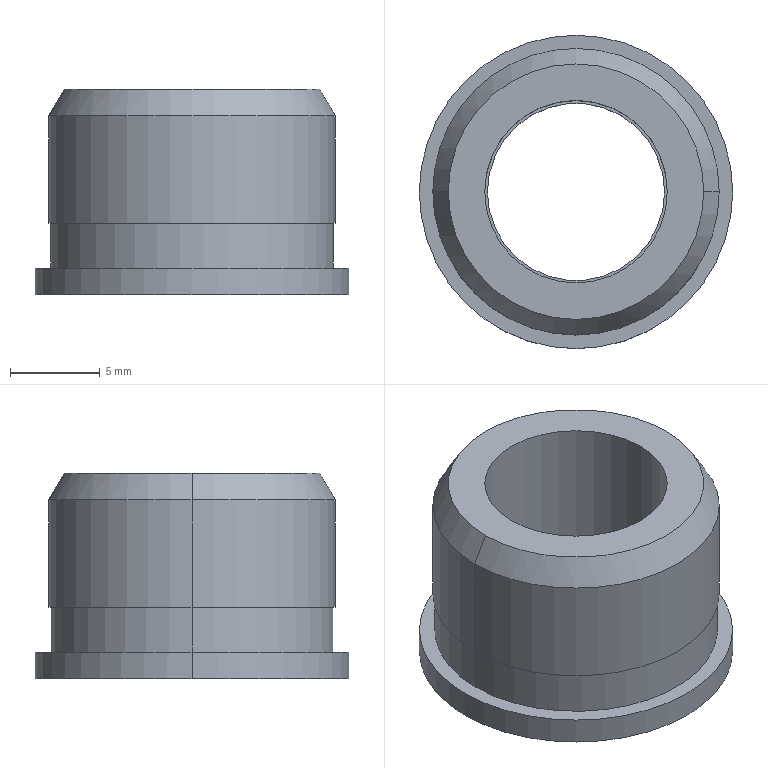Part | SolidWorks | features BaseBody 1 | 1 solid | 17 faces | box 17.5 x 17.5 x 11.5 mm | volume 1402 mm3 | cylinder 10 | plane 5 | cone 2 | commonest cylinder face diameters 9.9 x2 10.2 x2 15.8 x2 16 x2 17.5 x2
STEP:
#1=CARTESIAN_POINT('',(485.487,37.715,-16.134));
#2=VERTEX_POINT('',#1);
#3=CARTESIAN_POINT('',(475.587,37.715,-16.134));
#4=VERTEX_POINT('',#3);
#5=CARTESIAN_POINT('',(480.537,37.715,-16.134));
#6=DIRECTION('',(0.000000013,0.,-1.));
#7=DIRECTION('',(1.,0.,0.000000013));
#8=AXIS2_PLACEMENT_3D('',#5,#6,#7);
#9=CIRCLE('',#8,4.95);
#10=EDGE_CURVE('',#2,#4,#9,.T.);
#11=ORIENTED_EDGE('',*,*,#10,.T.);
#12=CARTESIAN_POINT('',(475.587,37.715,-13.134));
#13=VERTEX_POINT('',#12);
#14=CARTESIAN_POINT('',(475.587,37.715,-16.134));
#15=DIRECTION('',(-0.000000013,0.,1.));
#16=VECTOR('',#15,1000.);
#17=LINE('',#14,#16);
#18=EDGE_CURVE('',#4,#13,#17,.T.);
#19=ORIENTED_EDGE('',*,*,#18,.T.);
#20=CARTESIAN_POINT('',(485.487,37.715,-13.134));
#21=VERTEX_POINT('',#20);
#22=CARTESIAN_POINT('',(480.537,37.715,-13.134));
#23=DIRECTION('',(-0.000000013,0.,1.));
#24=DIRECTION('',(1.,0.,0.000000013));
#25=AXIS2_PLACEMENT_3D('',#22,#23,#24);
#26=CIRCLE('',#25,4.95);
#27=EDGE_CURVE('',#13,#21,#26,.T.);
#28=ORIENTED_EDGE('',*,*,#27,.T.);
#29=CARTESIAN_POINT('',(485.487,37.715,-16.134));
#30=DIRECTION('',(-0.000000013,0.,1.));
#31=VECTOR('',#30,1000.);
#32=LINE('',#29,#31);
#33=EDGE_CURVE('',#2,#21,#32,.T.);
#34=ORIENTED_EDGE('',*,*,#33,.F.);
#35=EDGE_LOOP('',(#11,#19,#28,#34));
#36=FACE_OUTER_BOUND('',#35,.T.);
#37=CARTESIAN_POINT('',(480.537,37.715,-16.134));
#38=DIRECTION('',(-0.000000013,0.,1.));
#39=DIRECTION('',(1.,0.,0.000000013));
#40=AXIS2_PLACEMENT_3D('',#37,#38,#39);
#41=CYLINDRICAL_SURFACE('',#40,4.95);
#42=ADVANCED_FACE('',(#36),#41,.F.);
#43=CARTESIAN_POINT('',(489.287,37.715,-16.134));
#44=VERTEX_POINT('',#43);
#45=CARTESIAN_POINT('',(471.787,37.715,-16.134));
#46=VERTEX_POINT('',#45);
#47=CARTESIAN_POINT('',(480.537,37.715,-16.134));
#48=DIRECTION('',(-0.000000013,0.,1.));
#49=DIRECTION('',(1.,0.,0.000000013));
#50=AXIS2_PLACEMENT_3D('',#47,#48,#49);
#51=CIRCLE('',#50,8.75);
#52=EDGE_CURVE('',#44,#46,#51,.T.);
#53=ORIENTED_EDGE('',*,*,#52,.T.);
#54=CARTESIAN_POINT('',(471.787,37.715,-14.634));
#55=VERTEX_POINT('',#54);
#56=CARTESIAN_POINT('',(471.787,37.715,-16.134));
#57=DIRECTION('',(-0.000000013,0.,1.));
#58=VECTOR('',#57,1000.);
#59=LINE('',#56,#58);
#60=EDGE_CURVE('',#46,#55,#59,.T.);
#61=ORIENTED_EDGE('',*,*,#60,.T.);
#62=CARTESIAN_POINT('',(489.287,37.715,-14.634));
#63=VERTEX_POINT('',#62);
#64=CARTESIAN_POINT('',(480.537,37.715,-14.634));
#65=DIRECTION('',(-0.000000013,0.,1.));
#66=DIRECTION('',(1.,0.,0.000000013));
#67=AXIS2_PLACEMENT_3D('',#64,#65,#66);
#68=CIRCLE('',#67,8.75);
#69=EDGE_CURVE('',#63,#55,#68,.T.);
#70=ORIENTED_EDGE('',*,*,#69,.F.);
#71=CARTESIAN_POINT('',(489.287,37.715,-16.134));
#72=DIRECTION('',(-0.000000013,0.,1.));
#73=VECTOR('',#72,1000.);
#74=LINE('',#71,#73);
#75=EDGE_CURVE('',#44,#63,#74,.T.);
#76=ORIENTED_EDGE('',*,*,#75,.F.);
#77=EDGE_LOOP('',(#53,#61,#70,#76));
#78=FACE_OUTER_BOUND('',#77,.T.);
#79=CARTESIAN_POINT('',(480.537,37.715,-16.134));
#80=DIRECTION('',(-0.000000013,0.,1.));
#81=DIRECTION('',(1.,0.,0.000000013));
#82=AXIS2_PLACEMENT_3D('',#79,#80,#81);
#83=CYLINDRICAL_SURFACE('',#82,8.75);
#84=ADVANCED_FACE('',(#78),#83,.T.);
#85=CARTESIAN_POINT('',(475.437,37.715,-13.134));
#86=VERTEX_POINT('',#85);
#87=CARTESIAN_POINT('',(485.637,37.715,-13.134));
#88=VERTEX_POINT('',#87);
#89=CARTESIAN_POINT('',(480.537,37.715,-13.134));
#90=DIRECTION('',(-0.000000013,0.,1.));
#91=DIRECTION('',(1.,0.,0.000000013));
#92=AXIS2_PLACEMENT_3D('',#89,#90,#91);
#93=CIRCLE('',#92,5.1);
#94=EDGE_CURVE('',#86,#88,#93,.T.);
#95=ORIENTED_EDGE('',*,*,#94,.F.);
#96=CARTESIAN_POINT('',(475.437,37.715,-4.634));
#97=VERTEX_POINT('',#96);
#98=CARTESIAN_POINT('',(475.437,37.715,-13.134));
#99=DIRECTION('',(-0.000000013,0.,1.));
#100=VECTOR('',#99,1000.);
#101=LINE('',#98,#100);
#102=EDGE_CURVE('',#86,#97,#101,.T.);
#103=ORIENTED_EDGE('',*,*,#102,.T.);
#104=CARTESIAN_POINT('',(485.637,37.715,-4.634));
#105=VERTEX_POINT('',#104);
#106=CARTESIAN_POINT('',(480.537,37.715,-4.634));
#107=DIRECTION('',(-0.000000013,0.,1.));
#108=DIRECTION('',(1.,0.,0.000000013));
#109=AXIS2_PLACEMENT_3D('',#106,#107,#108);
#110=CIRCLE('',#109,5.1);
#111=EDGE_CURVE('',#97,#105,#110,.T.);
#112=ORIENTED_EDGE('',*,*,#111,.T.);
#113=CARTESIAN_POINT('',(485.637,37.715,-13.134));
#114=DIRECTION('',(-0.000000013,0.,1.));
#115=VECTOR('',#114,1000.);
#116=LINE('',#113,#115);
#117=EDGE_CURVE('',#88,#105,#116,.T.);
#118=ORIENTED_EDGE('',*,*,#117,.F.);
#119=EDGE_LOOP('',(#95,#103,#112,#118));
#120=FACE_OUTER_BOUND('',#119,.T.);
#121=CARTESIAN_POINT('',(480.537,37.715,-13.134));
#122=DIRECTION('',(-0.000000013,0.,1.));
#123=DIRECTION('',(1.,0.,0.000000013));
#124=AXIS2_PLACEMENT_3D('',#121,#122,#123);
#125=CYLINDRICAL_SURFACE('',#124,5.1);
#126=ADVANCED_FACE('',(#120),#125,.F.);
#127=CARTESIAN_POINT('',(472.637,37.715,-14.634));
#128=VERTEX_POINT('',#127);
#129=CARTESIAN_POINT('',(488.437,37.715,-14.634));
#130=VERTEX_POINT('',#129);
#131=CARTESIAN_POINT('',(480.537,37.715,-14.634));
#132=DIRECTION('',(0.000000013,0.,-1.));
#133=DIRECTION('',(1.,0.,0.000000013));
#134=AXIS2_PLACEMENT_3D('',#131,#132,#133);
#135=CIRCLE('',#134,7.9);
#136=EDGE_CURVE('',#128,#130,#135,.T.);
#137=ORIENTED_EDGE('',*,*,#136,.F.);
#138=CARTESIAN_POINT('',(472.637,37.715,-12.134));
#139=VERTEX_POINT('',#138);
#140=CARTESIAN_POINT('',(472.637,37.715,-14.634));
#141=DIRECTION('',(-0.000000013,0.,1.));
#142=VECTOR('',#141,1000.);
#143=LINE('',#140,#142);
#144=EDGE_CURVE('',#128,#139,#143,.T.);
#145=ORIENTED_EDGE('',*,*,#144,.T.);
#146=CARTESIAN_POINT('',(488.437,37.715,-12.134));
#147=VERTEX_POINT('',#146);
#148=CARTESIAN_POINT('',(480.537,37.715,-12.134));
#149=DIRECTION('',(-0.000000013,0.,1.));
#150=DIRECTION('',(1.,0.,0.000000013));
#151=AXIS2_PLACEMENT_3D('',#148,#149,#150);
#152=CIRCLE('',#151,7.9);
#153=EDGE_CURVE('',#147,#139,#152,.T.);
#154=ORIENTED_EDGE('',*,*,#153,.F.);
#155=CARTESIAN_POINT('',(488.437,37.715,-14.634));
#156=DIRECTION('',(-0.000000013,0.,1.));
#157=VECTOR('',#156,1000.);
#158=LINE('',#155,#157);
#159=EDGE_CURVE('',#130,#147,#158,.T.);
#160=ORIENTED_EDGE('',*,*,#159,.F.);
#161=EDGE_LOOP('',(#137,#145,#154,#160));
#162=FACE_OUTER_BOUND('',#161,.T.);
#163=CARTESIAN_POINT('',(480.537,37.715,-14.634));
#164=DIRECTION('',(-0.000000013,0.,1.));
#165=DIRECTION('',(1.,0.,0.000000013));
#166=AXIS2_PLACEMENT_3D('',#163,#164,#165);
#167=CYLINDRICAL_SURFACE('',#166,7.9);
#168=ADVANCED_FACE('',(#162),#167,.T.);
#169=CARTESIAN_POINT('',(487.671,37.715,-4.634));
#170=VERTEX_POINT('',#169);
#171=CARTESIAN_POINT('',(473.403,37.715,-4.634));
#172=VERTEX_POINT('',#171);
#173=CARTESIAN_POINT('',(480.537,37.715,-4.634));
#174=DIRECTION('',(-0.000000013,0.,1.));
#175=DIRECTION('',(-1.,0.,-0.000000013));
#176=AXIS2_PLACEMENT_3D('',#173,#174,#175);
#177=CIRCLE('',#176,7.134);
#178=EDGE_CURVE('',#170,#172,#177,.T.);
#179=ORIENTED_EDGE('',*,*,#178,.F.);
#180=CARTESIAN_POINT('',(488.537,37.715,-6.134));
#181=VERTEX_POINT('',#180);
#182=CARTESIAN_POINT('',(488.537,37.715,-6.134));
#183=DIRECTION('',(0.5,0.,-0.866));
#184=VECTOR('',#183,1000.);
#185=LINE('',#182,#184);
#186=EDGE_CURVE('',#170,#181,#185,.T.);
#187=ORIENTED_EDGE('',*,*,#186,.T.);
#188=CARTESIAN_POINT('',(472.537,37.715,-6.134));
#189=VERTEX_POINT('',#188);
#190=CARTESIAN_POINT('',(480.537,37.715,-6.134));
#191=DIRECTION('',(0.000000013,0.,-1.));
#192=DIRECTION('',(0.,1.,0.));
#193=AXIS2_PLACEMENT_3D('',#190,#191,#192);
#194=CIRCLE('',#193,8.);
#195=EDGE_CURVE('',#189,#181,#194,.T.);
#196=ORIENTED_EDGE('',*,*,#195,.F.);
#197=CARTESIAN_POINT('',(472.537,37.715,-6.134));
#198=DIRECTION('',(-0.5,0.,-0.866));
#199=VECTOR('',#198,1000.);
#200=LINE('',#197,#199);
#201=EDGE_CURVE('',#172,#189,#200,.T.);
#202=ORIENTED_EDGE('',*,*,#201,.F.);
#203=EDGE_LOOP('',(#179,#187,#196,#202));
#204=FACE_OUTER_BOUND('',#203,.T.);
#205=CARTESIAN_POINT('',(480.537,37.715,-6.134));
#206=DIRECTION('',(0.000000013,0.,-1.));
#207=DIRECTION('',(-1.,0.,-0.000000013));
#208=AXIS2_PLACEMENT_3D('',#205,#206,#207);
#209=CONICAL_SURFACE('',#208,8.,0.5236);
#210=ADVANCED_FACE('',(#204),#209,.T.);
#211=CARTESIAN_POINT('',(488.537,37.715,-12.134));
#212=VERTEX_POINT('',#211);
#213=CARTESIAN_POINT('',(472.537,37.715,-12.134));
#214=VERTEX_POINT('',#213);
#215=CARTESIAN_POINT('',(480.537,37.715,-12.134));
#216=DIRECTION('',(-0.000000013,0.,1.));
#217=DIRECTION('',(1.,0.,0.000000013));
#218=AXIS2_PLACEMENT_3D('',#215,#216,#217);
#219=CIRCLE('',#218,8.);
#220=EDGE_CURVE('',#212,#214,#219,.T.);
#221=ORIENTED_EDGE('',*,*,#220,.T.);
#222=CARTESIAN_POINT('',(472.537,37.715,-12.134));
#223=DIRECTION('',(-0.000000013,0.,1.));
#224=VECTOR('',#223,1000.);
#225=LINE('',#222,#224);
#226=EDGE_CURVE('',#214,#189,#225,.T.);
#227=ORIENTED_EDGE('',*,*,#226,.T.);
#228=ORIENTED_EDGE('',*,*,#195,.T.);
#229=CARTESIAN_POINT('',(488.537,37.715,-12.134));
#230=DIRECTION('',(-0.000000013,0.,1.));
#231=VECTOR('',#230,1000.);
#232=LINE('',#229,#231);
#233=EDGE_CURVE('',#212,#181,#232,.T.);
#234=ORIENTED_EDGE('',*,*,#233,.F.);
#235=EDGE_LOOP('',(#221,#227,#228,#234));
#236=FACE_OUTER_BOUND('',#235,.T.);
#237=CARTESIAN_POINT('',(480.537,37.715,-12.134));
#238=DIRECTION('',(-0.000000013,0.,1.));
#239=DIRECTION('',(1.,0.,0.000000013));
#240=AXIS2_PLACEMENT_3D('',#237,#238,#239);
#241=CYLINDRICAL_SURFACE('',#240,8.);
#242=ADVANCED_FACE('',(#236),#241,.T.);
#243=ORIENTED_EDGE('',*,*,#10,.F.);
#244=CARTESIAN_POINT('',(480.537,37.715,-16.134));
#245=DIRECTION('',(0.000000013,0.,-1.));
#246=DIRECTION('',(1.,0.,0.000000013));
#247=AXIS2_PLACEMENT_3D('',#244,#245,#246);
#248=CIRCLE('',#247,4.95);
#249=EDGE_CURVE('',#4,#2,#248,.T.);
#250=ORIENTED_EDGE('',*,*,#249,.F.);
#251=EDGE_LOOP('',(#243,#250));
#252=FACE_BOUND('',#251,.T.);
#253=ORIENTED_EDGE('',*,*,#52,.F.);
#254=CARTESIAN_POINT('',(480.537,37.715,-16.134));
#255=DIRECTION('',(-0.000000013,0.,1.));
#256=DIRECTION('',(1.,0.,0.000000013));
#257=AXIS2_PLACEMENT_3D('',#254,#255,#256);
#258=CIRCLE('',#257,8.75);
#259=EDGE_CURVE('',#46,#44,#258,.T.);
#260=ORIENTED_EDGE('',*,*,#259,.F.);
#261=EDGE_LOOP('',(#253,#260));
#262=FACE_OUTER_BOUND('',#261,.T.);
#263=CARTESIAN_POINT('',(489.641,28.615,-16.134));
#264=DIRECTION('',(-0.000000013,0.,1.));
#265=DIRECTION('',(0.,1.,0.));
#266=AXIS2_PLACEMENT_3D('',#263,#264,#265);
#267=PLANE('',#266);
#268=ADVANCED_FACE('',(#252,#262),#267,.F.);
#269=ORIENTED_EDGE('',*,*,#18,.F.);
#270=ORIENTED_EDGE('',*,*,#249,.T.);
#271=ORIENTED_EDGE('',*,*,#33,.T.);
#272=CARTESIAN_POINT('',(480.537,37.715,-13.134));
#273=DIRECTION('',(-0.000000013,0.,1.));
#274=DIRECTION('',(1.,0.,0.000000013));
#275=AXIS2_PLACEMENT_3D('',#272,#273,#274);
#276=CIRCLE('',#275,4.95);
#277=EDGE_CURVE('',#21,#13,#276,.T.);
#278=ORIENTED_EDGE('',*,*,#277,.T.);
#279=EDGE_LOOP('',(#269,#270,#271,#278));
#280=FACE_OUTER_BOUND('',#279,.T.);
#281=CARTESIAN_POINT('',(480.537,37.715,-16.134));
#282=DIRECTION('',(-0.000000013,0.,1.));
#283=DIRECTION('',(1.,0.,0.000000013));
#284=AXIS2_PLACEMENT_3D('',#281,#282,#283);
#285=CYLINDRICAL_SURFACE('',#284,4.95);
#286=ADVANCED_FACE('',(#280),#285,.F.);
#287=ORIENTED_EDGE('',*,*,#60,.F.);
#288=ORIENTED_EDGE('',*,*,#259,.T.);
#289=ORIENTED_EDGE('',*,*,#75,.T.);
#290=CARTESIAN_POINT('',(480.537,37.715,-14.634));
#291=DIRECTION('',(-0.000000013,0.,1.));
#292=DIRECTION('',(1.,0.,0.000000013));
#293=AXIS2_PLACEMENT_3D('',#290,#291,#292);
#294=CIRCLE('',#293,8.75);
#295=EDGE_CURVE('',#55,#63,#294,.T.);
#296=ORIENTED_EDGE('',*,*,#295,.F.);
#297=EDGE_LOOP('',(#287,#288,#289,#296));
#298=FACE_OUTER_BOUND('',#297,.T.);
#299=CARTESIAN_POINT('',(480.537,37.715,-16.134));
#300=DIRECTION('',(-0.000000013,0.,1.));
#301=DIRECTION('',(1.,0.,0.000000013));
#302=AXIS2_PLACEMENT_3D('',#299,#300,#301);
#303=CYLINDRICAL_SURFACE('',#302,8.75);
#304=ADVANCED_FACE('',(#298),#303,.T.);
#305=ORIENTED_EDGE('',*,*,#277,.F.);
#306=ORIENTED_EDGE('',*,*,#27,.F.);
#307=EDGE_LOOP('',(#305,#306));
#308=FACE_BOUND('',#307,.T.);
#309=CARTESIAN_POINT('',(480.537,37.715,-13.134));
#310=DIRECTION('',(-0.000000013,0.,1.));
#311=DIRECTION('',(1.,0.,0.000000013));
#312=AXIS2_PLACEMENT_3D('',#309,#310,#311);
#313=CIRCLE('',#312,5.1);
#314=EDGE_CURVE('',#88,#86,#313,.T.);
#315=ORIENTED_EDGE('',*,*,#314,.T.);
#316=ORIENTED_EDGE('',*,*,#94,.T.);
#317=EDGE_LOOP('',(#315,#316));
#318=FACE_OUTER_BOUND('',#317,.T.);
#319=CARTESIAN_POINT('',(485.841,32.411,-13.134));
#320=DIRECTION('',(-0.000000013,0.,1.));
#321=DIRECTION('',(0.,1.,0.));
#322=AXIS2_PLACEMENT_3D('',#319,#320,#321);
#323=PLANE('',#322);
#324=ADVANCED_FACE('',(#308,#318),#323,.T.);
#325=CARTESIAN_POINT('',(480.537,37.715,-14.634));
#326=DIRECTION('',(0.000000013,0.,-1.));
#327=DIRECTION('',(1.,0.,0.000000013));
#328=AXIS2_PLACEMENT_3D('',#325,#326,#327);
#329=CIRCLE('',#328,7.9);
#330=EDGE_CURVE('',#130,#128,#329,.T.);
#331=ORIENTED_EDGE('',*,*,#330,.T.);
#332=ORIENTED_EDGE('',*,*,#136,.T.);
#333=EDGE_LOOP('',(#331,#332));
#334=FACE_BOUND('',#333,.T.);
#335=ORIENTED_EDGE('',*,*,#69,.T.);
#336=ORIENTED_EDGE('',*,*,#295,.T.);
#337=EDGE_LOOP('',(#335,#336));
#338=FACE_OUTER_BOUND('',#337,.T.);
#339=CARTESIAN_POINT('',(489.641,28.615,-14.634));
#340=DIRECTION('',(-0.000000013,0.,1.));
#341=DIRECTION('',(0.,1.,0.));
#342=AXIS2_PLACEMENT_3D('',#339,#340,#341);
#343=PLANE('',#342);
#344=ADVANCED_FACE('',(#334,#338),#343,.T.);
#345=ORIENTED_EDGE('',*,*,#102,.F.);
#346=ORIENTED_EDGE('',*,*,#314,.F.);
#347=ORIENTED_EDGE('',*,*,#117,.T.);
#348=CARTESIAN_POINT('',(480.537,37.715,-4.634));
#349=DIRECTION('',(-0.000000013,0.,1.));
#350=DIRECTION('',(1.,0.,0.000000013));
#351=AXIS2_PLACEMENT_3D('',#348,#349,#350);
#352=CIRCLE('',#351,5.1);
#353=EDGE_CURVE('',#105,#97,#352,.T.);
#354=ORIENTED_EDGE('',*,*,#353,.T.);
#355=EDGE_LOOP('',(#345,#346,#347,#354));
#356=FACE_OUTER_BOUND('',#355,.T.);
#357=CARTESIAN_POINT('',(480.537,37.715,-13.134));
#358=DIRECTION('',(-0.000000013,0.,1.));
#359=DIRECTION('',(1.,0.,0.000000013));
#360=AXIS2_PLACEMENT_3D('',#357,#358,#359);
#361=CYLINDRICAL_SURFACE('',#360,5.1);
#362=ADVANCED_FACE('',(#356),#361,.F.);
#363=ORIENTED_EDGE('',*,*,#144,.F.);
#364=ORIENTED_EDGE('',*,*,#330,.F.);
#365=ORIENTED_EDGE('',*,*,#159,.T.);
#366=CARTESIAN_POINT('',(480.537,37.715,-12.134));
#367=DIRECTION('',(-0.000000013,0.,1.));
#368=DIRECTION('',(1.,0.,0.000000013));
#369=AXIS2_PLACEMENT_3D('',#366,#367,#368);
#370=CIRCLE('',#369,7.9);
#371=EDGE_CURVE('',#139,#147,#370,.T.);
#372=ORIENTED_EDGE('',*,*,#371,.F.);
#373=EDGE_LOOP('',(#363,#364,#365,#372));
#374=FACE_OUTER_BOUND('',#373,.T.);
#375=CARTESIAN_POINT('',(480.537,37.715,-14.634));
#376=DIRECTION('',(-0.000000013,0.,1.));
#377=DIRECTION('',(1.,0.,0.000000013));
#378=AXIS2_PLACEMENT_3D('',#375,#376,#377);
#379=CYLINDRICAL_SURFACE('',#378,7.9);
#380=ADVANCED_FACE('',(#374),#379,.T.);
#381=ORIENTED_EDGE('',*,*,#353,.F.);
#382=ORIENTED_EDGE('',*,*,#111,.F.);
#383=EDGE_LOOP('',(#381,#382));
#384=FACE_BOUND('',#383,.T.);
#385=CARTESIAN_POINT('',(480.537,37.715,-4.634));
#386=DIRECTION('',(-0.000000013,0.,1.));
#387=DIRECTION('',(-1.,0.,-0.000000013));
#388=AXIS2_PLACEMENT_3D('',#385,#386,#387);
#389=CIRCLE('',#388,7.134);
#390=EDGE_CURVE('',#172,#170,#389,.T.);
#391=ORIENTED_EDGE('',*,*,#390,.T.);
#392=ORIENTED_EDGE('',*,*,#178,.T.);
#393=EDGE_LOOP('',(#391,#392));
#394=FACE_OUTER_BOUND('',#393,.T.);
#395=CARTESIAN_POINT('',(487.956,30.295,-4.634));
#396=DIRECTION('',(-0.000000013,0.,1.));
#397=DIRECTION('',(0.,1.,0.));
#398=AXIS2_PLACEMENT_3D('',#395,#396,#397);
#399=PLANE('',#398);
#400=ADVANCED_FACE('',(#384,#394),#399,.T.);
#401=ORIENTED_EDGE('',*,*,#153,.T.);
#402=ORIENTED_EDGE('',*,*,#371,.T.);
#403=EDGE_LOOP('',(#401,#402));
#404=FACE_BOUND('',#403,.T.);
#405=ORIENTED_EDGE('',*,*,#220,.F.);
#406=CARTESIAN_POINT('',(480.537,37.715,-12.134));
#407=DIRECTION('',(-0.000000013,0.,1.));
#408=DIRECTION('',(1.,0.,0.000000013));
#409=AXIS2_PLACEMENT_3D('',#406,#407,#408);
#410=CIRCLE('',#409,8.);
#411=EDGE_CURVE('',#214,#212,#410,.T.);
#412=ORIENTED_EDGE('',*,*,#411,.F.);
#413=EDGE_LOOP('',(#405,#412));
#414=FACE_OUTER_BOUND('',#413,.T.);
#415=CARTESIAN_POINT('',(488.857,29.395,-12.134));
#416=DIRECTION('',(-0.000000013,0.,1.));
#417=DIRECTION('',(0.,1.,0.));
#418=AXIS2_PLACEMENT_3D('',#415,#416,#417);
#419=PLANE('',#418);
#420=ADVANCED_FACE('',(#404,#414),#419,.F.);
#421=ORIENTED_EDGE('',*,*,#186,.F.);
#422=ORIENTED_EDGE('',*,*,#390,.F.);
#423=ORIENTED_EDGE('',*,*,#201,.T.);
#424=CARTESIAN_POINT('',(480.537,37.715,-6.134));
#425=DIRECTION('',(0.000000013,0.,-1.));
#426=DIRECTION('',(0.,1.,0.));
#427=AXIS2_PLACEMENT_3D('',#424,#425,#426);
#428=CIRCLE('',#427,8.);
#429=EDGE_CURVE('',#181,#189,#428,.T.);
#430=ORIENTED_EDGE('',*,*,#429,.F.);
#431=EDGE_LOOP('',(#421,#422,#423,#430));
#432=FACE_OUTER_BOUND('',#431,.T.);
#433=CARTESIAN_POINT('',(480.537,37.715,-6.134));
#434=DIRECTION('',(0.000000013,0.,-1.));
#435=DIRECTION('',(-1.,0.,-0.000000013));
#436=AXIS2_PLACEMENT_3D('',#433,#434,#435);
#437=CONICAL_SURFACE('',#436,8.,0.5236);
#438=ADVANCED_FACE('',(#432),#437,.T.);
#439=ORIENTED_EDGE('',*,*,#226,.F.);
#440=ORIENTED_EDGE('',*,*,#411,.T.);
#441=ORIENTED_EDGE('',*,*,#233,.T.);
#442=ORIENTED_EDGE('',*,*,#429,.T.);
#443=EDGE_LOOP('',(#439,#440,#441,#442));
#444=FACE_OUTER_BOUND('',#443,.T.);
#445=CARTESIAN_POINT('',(480.537,37.715,-12.134));
#446=DIRECTION('',(-0.000000013,0.,1.));
#447=DIRECTION('',(1.,0.,0.000000013));
#448=AXIS2_PLACEMENT_3D('',#445,#446,#447);
#449=CYLINDRICAL_SURFACE('',#448,8.);
#450=ADVANCED_FACE('',(#444),#449,.T.);
#451=CLOSED_SHELL('',(#42,#84,#126,#168,#210,#242,#268,#286,#304,#324,#344,#362,#380,#400,#420,#438,#450));
#452=MANIFOLD_SOLID_BREP('',#451);
#453=CARTESIAN_POINT('',(0.,0.,0.));
#454=DIRECTION('',(0.,0.,1.));
#455=DIRECTION('',(1.,0.,0.));
#456=AXIS2_PLACEMENT_3D('',#453,#454,#455);
#457=(LENGTH_UNIT()NAMED_UNIT(*)SI_UNIT(.MILLI.,.METRE.));
#458=UNCERTAINTY_MEASURE_WITH_UNIT(LENGTH_MEASURE(0.00001),#457,'','');
#459=(NAMED_UNIT(*)PLANE_ANGLE_UNIT()SI_UNIT($,.RADIAN.));
#460=(NAMED_UNIT(*)SI_UNIT($,.STERADIAN.)SOLID_ANGLE_UNIT());
#461=(GEOMETRIC_REPRESENTATION_CONTEXT(3)GLOBAL_UNCERTAINTY_ASSIGNED_CONTEXT((#458))GLOBAL_UNIT_ASSIGNED_CONTEXT((#457,#459,#460))REPRESENTATION_CONTEXT('',''));
#462=ADVANCED_BREP_SHAPE_REPRESENTATION('',(#452,#456),#461);